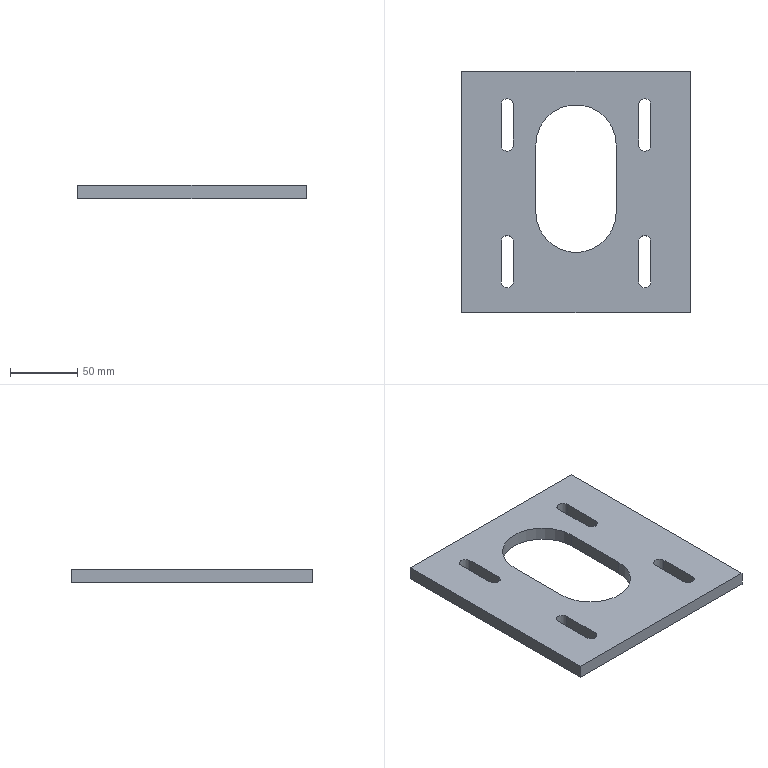Part | STEP file | 1 solid | 26 faces | box 170 x 180 x 10 mm | volume 234381 mm3 | plane 16 | cylinder 10 | commonest cylinder face diameters 9 x8 60 x2